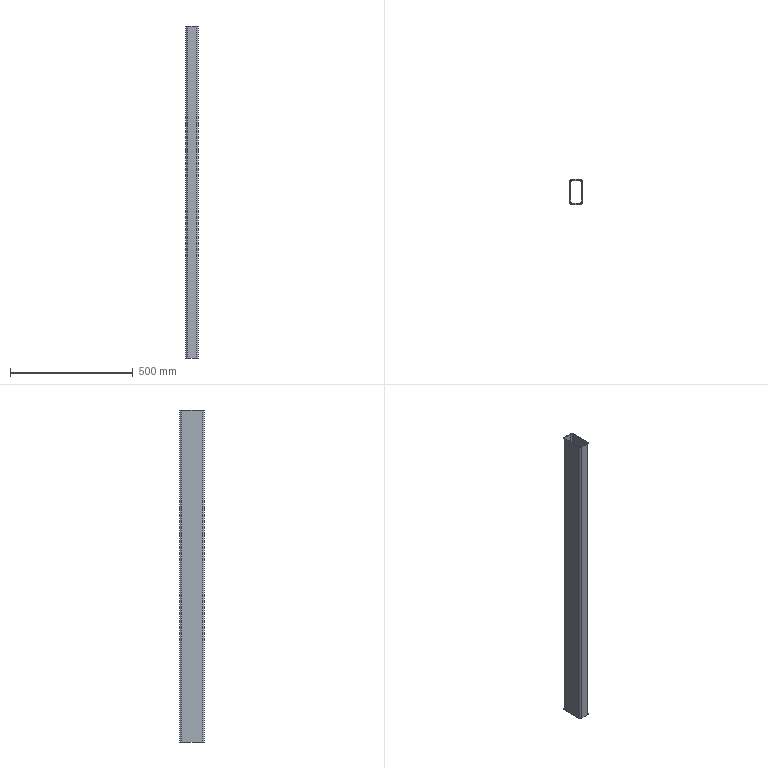Part | STEP file | KS D 3568 - 100 x 50 x 3.2 - 1350 | 1 solid | 18 faces | box 50 x 100 x 1350 mm | volume 1193238 mm3 | plane 10 | cylinder 8 | commonest cylinder face diameters 9.6 x4 16 x4
STEP:
#1=CARTESIAN_POINT('',(0.,0.,0.));
#2=DIRECTION('',(0.,0.,1.));
#3=DIRECTION('',(1.,0.,0.));
#4=AXIS2_PLACEMENT_3D('',#1,#2,#3);
#5=CARTESIAN_POINT('',(17.,46.8,1400.));
#6=VERTEX_POINT('',#5);
#7=CARTESIAN_POINT('',(-17.,46.8,1400.));
#8=VERTEX_POINT('',#7);
#9=CARTESIAN_POINT('',(-8.5,46.8,1400.));
#10=DIRECTION('',(-1.,0.,0.));
#11=VECTOR('',#10,1.);
#12=LINE('',#9,#11);
#13=CARTESIAN_POINT('',(0.,0.,1400.));
#14=DIRECTION('',(0.,0.,1.));
#15=DIRECTION('',(1.,0.,0.));
#16=AXIS2_PLACEMENT_3D('',#13,#14,#15);
#17=PLANE('',#16);
#18=CARTESIAN_POINT('',(-8.5,46.8));
#19=DIRECTION('',(-1.,0.));
#20=VECTOR('',#19,1.);
#21=LINE('',#18,#20);
#22=(GEOMETRIC_REPRESENTATION_CONTEXT(2)PARAMETRIC_REPRESENTATION_CONTEXT()REPRESENTATION_CONTEXT('',''));
#23=DEFINITIONAL_REPRESENTATION('',(#21),#22);
#24=PCURVE('',#17,#23);
#25=CARTESIAN_POINT('',(-17.,46.8,0.));
#26=DIRECTION('',(0.,1.,0.));
#27=DIRECTION('',(1.,0.,0.));
#28=AXIS2_PLACEMENT_3D('',#25,#26,#27);
#29=PLANE('',#28);
#30=CARTESIAN_POINT('',(8.5,-1400.));
#31=DIRECTION('',(-1.,0.));
#32=VECTOR('',#31,1.);
#33=LINE('',#30,#32);
#34=(GEOMETRIC_REPRESENTATION_CONTEXT(2)PARAMETRIC_REPRESENTATION_CONTEXT()REPRESENTATION_CONTEXT('',''));
#35=DEFINITIONAL_REPRESENTATION('',(#33),#34);
#36=PCURVE('',#29,#35);
#37=SURFACE_CURVE('',#12,(#24,#36),.PCURVE_S1.);
#38=EDGE_CURVE('',#6,#8,#37,.T.);
#39=ORIENTED_EDGE('',*,*,#38,.F.);
#40=CARTESIAN_POINT('',(21.8,42.,1400.));
#41=VERTEX_POINT('',#40);
#42=CARTESIAN_POINT('',(17.,42.,1400.));
#43=DIRECTION('',(0.,0.,1.));
#44=DIRECTION('',(-1.,0.,0.));
#45=AXIS2_PLACEMENT_3D('',#42,#43,#44);
#46=CIRCLE('',#45,4.8);
#47=CARTESIAN_POINT('',(17.,42.));
#48=DIRECTION('',(-1.,0.));
#49=AXIS2_PLACEMENT_2D('',#47,#48);
#50=CIRCLE('',#49,4.8);
#51=(GEOMETRIC_REPRESENTATION_CONTEXT(2)PARAMETRIC_REPRESENTATION_CONTEXT()REPRESENTATION_CONTEXT('',''));
#52=DEFINITIONAL_REPRESENTATION('',(#50),#51);
#53=PCURVE('',#17,#52);
#54=CARTESIAN_POINT('',(17.,42.,0.));
#55=DIRECTION('',(0.,0.,1.));
#56=DIRECTION('',(-1.,0.,0.));
#57=AXIS2_PLACEMENT_3D('',#54,#55,#56);
#58=CYLINDRICAL_SURFACE('',#57,4.8);
#59=CARTESIAN_POINT('',(0.,1400.));
#60=DIRECTION('',(1.,0.));
#61=VECTOR('',#60,1.);
#62=LINE('',#59,#61);
#63=(GEOMETRIC_REPRESENTATION_CONTEXT(2)PARAMETRIC_REPRESENTATION_CONTEXT()REPRESENTATION_CONTEXT('',''));
#64=DEFINITIONAL_REPRESENTATION('',(#62),#63);
#65=PCURVE('',#58,#64);
#66=SURFACE_CURVE('',#46,(#53,#65),.PCURVE_S1.);
#67=EDGE_CURVE('',#41,#6,#66,.T.);
#68=ORIENTED_EDGE('',*,*,#67,.F.);
#69=CARTESIAN_POINT('',(21.8,-42.,1400.));
#70=VERTEX_POINT('',#69);
#71=CARTESIAN_POINT('',(21.8,21.,1400.));
#72=DIRECTION('',(0.,1.,0.));
#73=VECTOR('',#72,1.);
#74=LINE('',#71,#73);
#75=CARTESIAN_POINT('',(21.8,21.));
#76=DIRECTION('',(0.,1.));
#77=VECTOR('',#76,1.);
#78=LINE('',#75,#77);
#79=(GEOMETRIC_REPRESENTATION_CONTEXT(2)PARAMETRIC_REPRESENTATION_CONTEXT()REPRESENTATION_CONTEXT('',''));
#80=DEFINITIONAL_REPRESENTATION('',(#78),#79);
#81=PCURVE('',#17,#80);
#82=CARTESIAN_POINT('',(21.8,42.,0.));
#83=DIRECTION('',(1.,0.,0.));
#84=DIRECTION('',(0.,1.,0.));
#85=AXIS2_PLACEMENT_3D('',#82,#83,#84);
#86=PLANE('',#85);
#87=CARTESIAN_POINT('',(-21.,1400.));
#88=DIRECTION('',(1.,0.));
#89=VECTOR('',#88,1.);
#90=LINE('',#87,#89);
#91=(GEOMETRIC_REPRESENTATION_CONTEXT(2)PARAMETRIC_REPRESENTATION_CONTEXT()REPRESENTATION_CONTEXT('',''));
#92=DEFINITIONAL_REPRESENTATION('',(#90),#91);
#93=PCURVE('',#86,#92);
#94=SURFACE_CURVE('',#74,(#81,#93),.PCURVE_S1.);
#95=EDGE_CURVE('',#70,#41,#94,.T.);
#96=ORIENTED_EDGE('',*,*,#95,.F.);
#97=CARTESIAN_POINT('',(17.,-46.8,1400.));
#98=VERTEX_POINT('',#97);
#99=CARTESIAN_POINT('',(17.,-42.,1400.));
#100=DIRECTION('',(0.,0.,1.));
#101=DIRECTION('',(0.,1.,0.));
#102=AXIS2_PLACEMENT_3D('',#99,#100,#101);
#103=CIRCLE('',#102,4.8);
#104=CARTESIAN_POINT('',(17.,-42.));
#105=DIRECTION('',(0.,1.));
#106=AXIS2_PLACEMENT_2D('',#104,#105);
#107=CIRCLE('',#106,4.8);
#108=(GEOMETRIC_REPRESENTATION_CONTEXT(2)PARAMETRIC_REPRESENTATION_CONTEXT()REPRESENTATION_CONTEXT('',''));
#109=DEFINITIONAL_REPRESENTATION('',(#107),#108);
#110=PCURVE('',#17,#109);
#111=CARTESIAN_POINT('',(17.,-42.,0.));
#112=DIRECTION('',(0.,0.,1.));
#113=DIRECTION('',(0.,1.,0.));
#114=AXIS2_PLACEMENT_3D('',#111,#112,#113);
#115=CYLINDRICAL_SURFACE('',#114,4.8);
#116=CARTESIAN_POINT('',(0.,1400.));
#117=DIRECTION('',(1.,0.));
#118=VECTOR('',#117,1.);
#119=LINE('',#116,#118);
#120=(GEOMETRIC_REPRESENTATION_CONTEXT(2)PARAMETRIC_REPRESENTATION_CONTEXT()REPRESENTATION_CONTEXT('',''));
#121=DEFINITIONAL_REPRESENTATION('',(#119),#120);
#122=PCURVE('',#115,#121);
#123=SURFACE_CURVE('',#103,(#110,#122),.PCURVE_S1.);
#124=EDGE_CURVE('',#98,#70,#123,.T.);
#125=ORIENTED_EDGE('',*,*,#124,.F.);
#126=CARTESIAN_POINT('',(-17.,-46.8,1400.));
#127=VERTEX_POINT('',#126);
#128=CARTESIAN_POINT('',(8.5,-46.8,1400.));
#129=DIRECTION('',(1.,0.,0.));
#130=VECTOR('',#129,1.);
#131=LINE('',#128,#130);
#132=CARTESIAN_POINT('',(8.5,-46.8));
#133=DIRECTION('',(1.,0.));
#134=VECTOR('',#133,1.);
#135=LINE('',#132,#134);
#136=(GEOMETRIC_REPRESENTATION_CONTEXT(2)PARAMETRIC_REPRESENTATION_CONTEXT()REPRESENTATION_CONTEXT('',''));
#137=DEFINITIONAL_REPRESENTATION('',(#135),#136);
#138=PCURVE('',#17,#137);
#139=CARTESIAN_POINT('',(17.,-46.8,0.));
#140=DIRECTION('',(0.,-1.,0.));
#141=DIRECTION('',(0.,0.,-1.));
#142=AXIS2_PLACEMENT_3D('',#139,#140,#141);
#143=PLANE('',#142);
#144=CARTESIAN_POINT('',(-1400.,-8.5));
#145=DIRECTION('',(0.,1.));
#146=VECTOR('',#145,1.);
#147=LINE('',#144,#146);
#148=(GEOMETRIC_REPRESENTATION_CONTEXT(2)PARAMETRIC_REPRESENTATION_CONTEXT()REPRESENTATION_CONTEXT('',''));
#149=DEFINITIONAL_REPRESENTATION('',(#147),#148);
#150=PCURVE('',#143,#149);
#151=SURFACE_CURVE('',#131,(#138,#150),.PCURVE_S1.);
#152=EDGE_CURVE('',#127,#98,#151,.T.);
#153=ORIENTED_EDGE('',*,*,#152,.F.);
#154=CARTESIAN_POINT('',(-21.8,-42.,1400.));
#155=VERTEX_POINT('',#154);
#156=CARTESIAN_POINT('',(-17.,-42.,1400.));
#157=DIRECTION('',(0.,0.,1.));
#158=DIRECTION('',(1.,0.,0.));
#159=AXIS2_PLACEMENT_3D('',#156,#157,#158);
#160=CIRCLE('',#159,4.8);
#161=CARTESIAN_POINT('',(-17.,-42.));
#162=DIRECTION('',(1.,0.));
#163=AXIS2_PLACEMENT_2D('',#161,#162);
#164=CIRCLE('',#163,4.8);
#165=(GEOMETRIC_REPRESENTATION_CONTEXT(2)PARAMETRIC_REPRESENTATION_CONTEXT()REPRESENTATION_CONTEXT('',''));
#166=DEFINITIONAL_REPRESENTATION('',(#164),#165);
#167=PCURVE('',#17,#166);
#168=CARTESIAN_POINT('',(-17.,-42.,0.));
#169=DIRECTION('',(0.,0.,1.));
#170=DIRECTION('',(1.,0.,0.));
#171=AXIS2_PLACEMENT_3D('',#168,#169,#170);
#172=CYLINDRICAL_SURFACE('',#171,4.8);
#173=CARTESIAN_POINT('',(0.,1400.));
#174=DIRECTION('',(1.,0.));
#175=VECTOR('',#174,1.);
#176=LINE('',#173,#175);
#177=(GEOMETRIC_REPRESENTATION_CONTEXT(2)PARAMETRIC_REPRESENTATION_CONTEXT()REPRESENTATION_CONTEXT('',''));
#178=DEFINITIONAL_REPRESENTATION('',(#176),#177);
#179=PCURVE('',#172,#178);
#180=SURFACE_CURVE('',#160,(#167,#179),.PCURVE_S1.);
#181=EDGE_CURVE('',#155,#127,#180,.T.);
#182=ORIENTED_EDGE('',*,*,#181,.F.);
#183=CARTESIAN_POINT('',(-21.8,42.,1400.));
#184=VERTEX_POINT('',#183);
#185=CARTESIAN_POINT('',(-21.8,-21.,1400.));
#186=DIRECTION('',(0.,-1.,0.));
#187=VECTOR('',#186,1.);
#188=LINE('',#185,#187);
#189=CARTESIAN_POINT('',(-21.8,-21.));
#190=DIRECTION('',(0.,-1.));
#191=VECTOR('',#190,1.);
#192=LINE('',#189,#191);
#193=(GEOMETRIC_REPRESENTATION_CONTEXT(2)PARAMETRIC_REPRESENTATION_CONTEXT()REPRESENTATION_CONTEXT('',''));
#194=DEFINITIONAL_REPRESENTATION('',(#192),#193);
#195=PCURVE('',#17,#194);
#196=CARTESIAN_POINT('',(-21.8,-42.,0.));
#197=DIRECTION('',(-1.,0.,0.));
#198=DIRECTION('',(0.,1.,0.));
#199=AXIS2_PLACEMENT_3D('',#196,#197,#198);
#200=PLANE('',#199);
#201=CARTESIAN_POINT('',(21.,-1400.));
#202=DIRECTION('',(-1.,0.));
#203=VECTOR('',#202,1.);
#204=LINE('',#201,#203);
#205=(GEOMETRIC_REPRESENTATION_CONTEXT(2)PARAMETRIC_REPRESENTATION_CONTEXT()REPRESENTATION_CONTEXT('',''));
#206=DEFINITIONAL_REPRESENTATION('',(#204),#205);
#207=PCURVE('',#200,#206);
#208=SURFACE_CURVE('',#188,(#195,#207),.PCURVE_S1.);
#209=EDGE_CURVE('',#184,#155,#208,.T.);
#210=ORIENTED_EDGE('',*,*,#209,.F.);
#211=CARTESIAN_POINT('',(-17.,42.,1400.));
#212=DIRECTION('',(0.,0.,1.));
#213=DIRECTION('',(0.,-1.,0.));
#214=AXIS2_PLACEMENT_3D('',#211,#212,#213);
#215=CIRCLE('',#214,4.8);
#216=CARTESIAN_POINT('',(-17.,42.));
#217=DIRECTION('',(0.,-1.));
#218=AXIS2_PLACEMENT_2D('',#216,#217);
#219=CIRCLE('',#218,4.8);
#220=(GEOMETRIC_REPRESENTATION_CONTEXT(2)PARAMETRIC_REPRESENTATION_CONTEXT()REPRESENTATION_CONTEXT('',''));
#221=DEFINITIONAL_REPRESENTATION('',(#219),#220);
#222=PCURVE('',#17,#221);
#223=CARTESIAN_POINT('',(-17.,42.,0.));
#224=DIRECTION('',(0.,0.,1.));
#225=DIRECTION('',(0.,-1.,0.));
#226=AXIS2_PLACEMENT_3D('',#223,#224,#225);
#227=CYLINDRICAL_SURFACE('',#226,4.8);
#228=CARTESIAN_POINT('',(0.,1400.));
#229=DIRECTION('',(1.,0.));
#230=VECTOR('',#229,1.);
#231=LINE('',#228,#230);
#232=(GEOMETRIC_REPRESENTATION_CONTEXT(2)PARAMETRIC_REPRESENTATION_CONTEXT()REPRESENTATION_CONTEXT('',''));
#233=DEFINITIONAL_REPRESENTATION('',(#231),#232);
#234=PCURVE('',#227,#233);
#235=SURFACE_CURVE('',#215,(#222,#234),.PCURVE_S1.);
#236=EDGE_CURVE('',#8,#184,#235,.T.);
#237=ORIENTED_EDGE('',*,*,#236,.F.);
#238=EDGE_LOOP('',(#39,#68,#96,#125,#153,#182,#210,#237));
#239=FACE_BOUND('',#238,.T.);
#240=CARTESIAN_POINT('',(-25.,-42.,1400.));
#241=VERTEX_POINT('',#240);
#242=CARTESIAN_POINT('',(-25.,42.,1400.));
#243=VERTEX_POINT('',#242);
#244=CARTESIAN_POINT('',(-25.,-21.,1400.));
#245=DIRECTION('',(0.,1.,0.));
#246=VECTOR('',#245,1.);
#247=LINE('',#244,#246);
#248=CARTESIAN_POINT('',(-25.,-21.));
#249=DIRECTION('',(0.,1.));
#250=VECTOR('',#249,1.);
#251=LINE('',#248,#250);
#252=(GEOMETRIC_REPRESENTATION_CONTEXT(2)PARAMETRIC_REPRESENTATION_CONTEXT()REPRESENTATION_CONTEXT('',''));
#253=DEFINITIONAL_REPRESENTATION('',(#251),#252);
#254=PCURVE('',#17,#253);
#255=CARTESIAN_POINT('',(-25.,-42.,0.));
#256=DIRECTION('',(-1.,0.,0.));
#257=DIRECTION('',(0.,1.,0.));
#258=AXIS2_PLACEMENT_3D('',#255,#256,#257);
#259=PLANE('',#258);
#260=CARTESIAN_POINT('',(21.,-1400.));
#261=DIRECTION('',(1.,0.));
#262=VECTOR('',#261,1.);
#263=LINE('',#260,#262);
#264=(GEOMETRIC_REPRESENTATION_CONTEXT(2)PARAMETRIC_REPRESENTATION_CONTEXT()REPRESENTATION_CONTEXT('',''));
#265=DEFINITIONAL_REPRESENTATION('',(#263),#264);
#266=PCURVE('',#259,#265);
#267=SURFACE_CURVE('',#247,(#254,#266),.PCURVE_S1.);
#268=EDGE_CURVE('',#241,#243,#267,.T.);
#269=ORIENTED_EDGE('',*,*,#268,.F.);
#270=CARTESIAN_POINT('',(-17.,-50.,1400.));
#271=VERTEX_POINT('',#270);
#272=CARTESIAN_POINT('',(-17.,-42.,1400.));
#273=DIRECTION('',(0.,0.,-1.));
#274=DIRECTION('',(1.,0.,0.));
#275=AXIS2_PLACEMENT_3D('',#272,#273,#274);
#276=CIRCLE('',#275,8.);
#277=CARTESIAN_POINT('',(-9.,-42.));
#278=CARTESIAN_POINT('',(-9.,-55.856));
#279=CARTESIAN_POINT('',(-21.,-48.928));
#280=CARTESIAN_POINT('',(-33.,-42.));
#281=CARTESIAN_POINT('',(-21.,-35.072));
#282=CARTESIAN_POINT('',(-9.,-28.144));
#283=CARTESIAN_POINT('',(-9.,-42.));
#284=(BOUNDED_CURVE()B_SPLINE_CURVE(2,(#277,#278,#279,#280,#281,#282,#283),.UNSPECIFIED.,.T.,.F.)B_SPLINE_CURVE_WITH_KNOTS((1,2,2,2,2,1),(-2.094,0.,2.094,4.189,6.283,8.378),.UNSPECIFIED.)CURVE()GEOMETRIC_REPRESENTATION_ITEM()RATIONAL_B_SPLINE_CURVE((1.,0.5,1.,0.5,1.,0.5,1.))REPRESENTATION_ITEM(''));
#285=(GEOMETRIC_REPRESENTATION_CONTEXT(2)PARAMETRIC_REPRESENTATION_CONTEXT()REPRESENTATION_CONTEXT('',''));
#286=DEFINITIONAL_REPRESENTATION('',(#284),#285);
#287=PCURVE('',#17,#286);
#288=CARTESIAN_POINT('',(-17.,-42.,0.));
#289=DIRECTION('',(0.,0.,1.));
#290=DIRECTION('',(1.,0.,0.));
#291=AXIS2_PLACEMENT_3D('',#288,#289,#290);
#292=CYLINDRICAL_SURFACE('',#291,8.);
#293=CARTESIAN_POINT('',(6.283,1400.));
#294=DIRECTION('',(-1.,0.));
#295=VECTOR('',#294,1.);
#296=LINE('',#293,#295);
#297=(GEOMETRIC_REPRESENTATION_CONTEXT(2)PARAMETRIC_REPRESENTATION_CONTEXT()REPRESENTATION_CONTEXT('',''));
#298=DEFINITIONAL_REPRESENTATION('',(#296),#297);
#299=PCURVE('',#292,#298);
#300=SURFACE_CURVE('',#276,(#287,#299),.PCURVE_S1.);
#301=EDGE_CURVE('',#271,#241,#300,.T.);
#302=ORIENTED_EDGE('',*,*,#301,.F.);
#303=CARTESIAN_POINT('',(17.,-50.,1400.));
#304=VERTEX_POINT('',#303);
#305=CARTESIAN_POINT('',(8.5,-50.,1400.));
#306=DIRECTION('',(-1.,0.,0.));
#307=VECTOR('',#306,1.);
#308=LINE('',#305,#307);
#309=CARTESIAN_POINT('',(8.5,-50.));
#310=DIRECTION('',(-1.,0.));
#311=VECTOR('',#310,1.);
#312=LINE('',#309,#311);
#313=(GEOMETRIC_REPRESENTATION_CONTEXT(2)PARAMETRIC_REPRESENTATION_CONTEXT()REPRESENTATION_CONTEXT('',''));
#314=DEFINITIONAL_REPRESENTATION('',(#312),#313);
#315=PCURVE('',#17,#314);
#316=CARTESIAN_POINT('',(17.,-50.,0.));
#317=DIRECTION('',(0.,-1.,0.));
#318=DIRECTION('',(-1.,0.,0.));
#319=AXIS2_PLACEMENT_3D('',#316,#317,#318);
#320=PLANE('',#319);
#321=CARTESIAN_POINT('',(8.5,-1400.));
#322=DIRECTION('',(1.,0.));
#323=VECTOR('',#322,1.);
#324=LINE('',#321,#323);
#325=(GEOMETRIC_REPRESENTATION_CONTEXT(2)PARAMETRIC_REPRESENTATION_CONTEXT()REPRESENTATION_CONTEXT('',''));
#326=DEFINITIONAL_REPRESENTATION('',(#324),#325);
#327=PCURVE('',#320,#326);
#328=SURFACE_CURVE('',#308,(#315,#327),.PCURVE_S1.);
#329=EDGE_CURVE('',#304,#271,#328,.T.);
#330=ORIENTED_EDGE('',*,*,#329,.F.);
#331=CARTESIAN_POINT('',(25.,-42.,1400.));
#332=VERTEX_POINT('',#331);
#333=CARTESIAN_POINT('',(17.,-42.,1400.));
#334=DIRECTION('',(0.,0.,-1.));
#335=DIRECTION('',(0.,1.,0.));
#336=AXIS2_PLACEMENT_3D('',#333,#334,#335);
#337=CIRCLE('',#336,8.);
#338=CARTESIAN_POINT('',(17.,-34.));
#339=CARTESIAN_POINT('',(30.856,-34.));
#340=CARTESIAN_POINT('',(23.928,-46.));
#341=CARTESIAN_POINT('',(17.,-58.));
#342=CARTESIAN_POINT('',(10.072,-46.));
#343=CARTESIAN_POINT('',(3.144,-34.));
#344=CARTESIAN_POINT('',(17.,-34.));
#345=(BOUNDED_CURVE()B_SPLINE_CURVE(2,(#338,#339,#340,#341,#342,#343,#344),.UNSPECIFIED.,.T.,.F.)B_SPLINE_CURVE_WITH_KNOTS((1,2,2,2,2,1),(-2.094,0.,2.094,4.189,6.283,8.378),.UNSPECIFIED.)CURVE()GEOMETRIC_REPRESENTATION_ITEM()RATIONAL_B_SPLINE_CURVE((1.,0.5,1.,0.5,1.,0.5,1.))REPRESENTATION_ITEM(''));
#346=(GEOMETRIC_REPRESENTATION_CONTEXT(2)PARAMETRIC_REPRESENTATION_CONTEXT()REPRESENTATION_CONTEXT('',''));
#347=DEFINITIONAL_REPRESENTATION('',(#345),#346);
#348=PCURVE('',#17,#347);
#349=CARTESIAN_POINT('',(17.,-42.,0.));
#350=DIRECTION('',(0.,0.,1.));
#351=DIRECTION('',(0.,1.,0.));
#352=AXIS2_PLACEMENT_3D('',#349,#350,#351);
#353=CYLINDRICAL_SURFACE('',#352,8.);
#354=CARTESIAN_POINT('',(6.283,1400.));
#355=DIRECTION('',(-1.,0.));
#356=VECTOR('',#355,1.);
#357=LINE('',#354,#356);
#358=(GEOMETRIC_REPRESENTATION_CONTEXT(2)PARAMETRIC_REPRESENTATION_CONTEXT()REPRESENTATION_CONTEXT('',''));
#359=DEFINITIONAL_REPRESENTATION('',(#357),#358);
#360=PCURVE('',#353,#359);
#361=SURFACE_CURVE('',#337,(#348,#360),.PCURVE_S1.);
#362=EDGE_CURVE('',#332,#304,#361,.T.);
#363=ORIENTED_EDGE('',*,*,#362,.F.);
#364=CARTESIAN_POINT('',(25.,42.,1400.));
#365=VERTEX_POINT('',#364);
#366=CARTESIAN_POINT('',(25.,21.,1400.));
#367=DIRECTION('',(0.,-1.,0.));
#368=VECTOR('',#367,1.);
#369=LINE('',#366,#368);
#370=CARTESIAN_POINT('',(25.,21.));
#371=DIRECTION('',(0.,-1.));
#372=VECTOR('',#371,1.);
#373=LINE('',#370,#372);
#374=(GEOMETRIC_REPRESENTATION_CONTEXT(2)PARAMETRIC_REPRESENTATION_CONTEXT()REPRESENTATION_CONTEXT('',''));
#375=DEFINITIONAL_REPRESENTATION('',(#373),#374);
#376=PCURVE('',#17,#375);
#377=CARTESIAN_POINT('',(25.,42.,0.));
#378=DIRECTION('',(1.,0.,0.));
#379=DIRECTION('',(0.,-1.,0.));
#380=AXIS2_PLACEMENT_3D('',#377,#378,#379);
#381=PLANE('',#380);
#382=CARTESIAN_POINT('',(21.,-1400.));
#383=DIRECTION('',(1.,0.));
#384=VECTOR('',#383,1.);
#385=LINE('',#382,#384);
#386=(GEOMETRIC_REPRESENTATION_CONTEXT(2)PARAMETRIC_REPRESENTATION_CONTEXT()REPRESENTATION_CONTEXT('',''));
#387=DEFINITIONAL_REPRESENTATION('',(#385),#386);
#388=PCURVE('',#381,#387);
#389=SURFACE_CURVE('',#369,(#376,#388),.PCURVE_S1.);
#390=EDGE_CURVE('',#365,#332,#389,.T.);
#391=ORIENTED_EDGE('',*,*,#390,.F.);
#392=CARTESIAN_POINT('',(17.,50.,1400.));
#393=VERTEX_POINT('',#392);
#394=CARTESIAN_POINT('',(17.,42.,1400.));
#395=DIRECTION('',(0.,0.,-1.));
#396=DIRECTION('',(-1.,0.,0.));
#397=AXIS2_PLACEMENT_3D('',#394,#395,#396);
#398=CIRCLE('',#397,8.);
#399=CARTESIAN_POINT('',(9.,42.));
#400=CARTESIAN_POINT('',(9.,55.856));
#401=CARTESIAN_POINT('',(21.,48.928));
#402=CARTESIAN_POINT('',(33.,42.));
#403=CARTESIAN_POINT('',(21.,35.072));
#404=CARTESIAN_POINT('',(9.,28.144));
#405=CARTESIAN_POINT('',(9.,42.));
#406=(BOUNDED_CURVE()B_SPLINE_CURVE(2,(#399,#400,#401,#402,#403,#404,#405),.UNSPECIFIED.,.T.,.F.)B_SPLINE_CURVE_WITH_KNOTS((1,2,2,2,2,1),(-2.094,0.,2.094,4.189,6.283,8.378),.UNSPECIFIED.)CURVE()GEOMETRIC_REPRESENTATION_ITEM()RATIONAL_B_SPLINE_CURVE((1.,0.5,1.,0.5,1.,0.5,1.))REPRESENTATION_ITEM(''));
#407=(GEOMETRIC_REPRESENTATION_CONTEXT(2)PARAMETRIC_REPRESENTATION_CONTEXT()REPRESENTATION_CONTEXT('',''));
#408=DEFINITIONAL_REPRESENTATION('',(#406),#407);
#409=PCURVE('',#17,#408);
#410=CARTESIAN_POINT('',(17.,42.,0.));
#411=DIRECTION('',(0.,0.,1.));
#412=DIRECTION('',(-1.,0.,0.));
#413=AXIS2_PLACEMENT_3D('',#410,#411,#412);
#414=CYLINDRICAL_SURFACE('',#413,8.);
#415=CARTESIAN_POINT('',(6.283,1400.));
#416=DIRECTION('',(-1.,0.));
#417=VECTOR('',#416,1.);
#418=LINE('',#415,#417);
#419=(GEOMETRIC_REPRESENTATION_CONTEXT(2)PARAMETRIC_REPRESENTATION_CONTEXT()REPRESENTATION_CONTEXT('',''));
#420=DEFINITIONAL_REPRESENTATION('',(#418),#419);
#421=PCURVE('',#414,#420);
#422=SURFACE_CURVE('',#398,(#409,#421),.PCURVE_S1.);
#423=EDGE_CURVE('',#393,#365,#422,.T.);
#424=ORIENTED_EDGE('',*,*,#423,.F.);
#425=CARTESIAN_POINT('',(-17.,50.,1400.));
#426=VERTEX_POINT('',#425);
#427=CARTESIAN_POINT('',(-8.5,50.,1400.));
#428=DIRECTION('',(1.,0.,0.));
#429=VECTOR('',#428,1.);
#430=LINE('',#427,#429);
#431=CARTESIAN_POINT('',(-8.5,50.));
#432=DIRECTION('',(1.,0.));
#433=VECTOR('',#432,1.);
#434=LINE('',#431,#433);
#435=(GEOMETRIC_REPRESENTATION_CONTEXT(2)PARAMETRIC_REPRESENTATION_CONTEXT()REPRESENTATION_CONTEXT('',''));
#436=DEFINITIONAL_REPRESENTATION('',(#434),#435);
#437=PCURVE('',#17,#436);
#438=CARTESIAN_POINT('',(-17.,50.,0.));
#439=DIRECTION('',(0.,1.,0.));
#440=DIRECTION('',(1.,0.,0.));
#441=AXIS2_PLACEMENT_3D('',#438,#439,#440);
#442=PLANE('',#441);
#443=CARTESIAN_POINT('',(8.5,-1400.));
#444=DIRECTION('',(1.,0.));
#445=VECTOR('',#444,1.);
#446=LINE('',#443,#445);
#447=(GEOMETRIC_REPRESENTATION_CONTEXT(2)PARAMETRIC_REPRESENTATION_CONTEXT()REPRESENTATION_CONTEXT('',''));
#448=DEFINITIONAL_REPRESENTATION('',(#446),#447);
#449=PCURVE('',#442,#448);
#450=SURFACE_CURVE('',#430,(#437,#449),.PCURVE_S1.);
#451=EDGE_CURVE('',#426,#393,#450,.T.);
#452=ORIENTED_EDGE('',*,*,#451,.F.);
#453=CARTESIAN_POINT('',(-17.,42.,1400.));
#454=DIRECTION('',(0.,0.,-1.));
#455=DIRECTION('',(0.,-1.,0.));
#456=AXIS2_PLACEMENT_3D('',#453,#454,#455);
#457=CIRCLE('',#456,8.);
#458=CARTESIAN_POINT('',(-17.,34.));
#459=CARTESIAN_POINT('',(-30.856,34.));
#460=CARTESIAN_POINT('',(-23.928,46.));
#461=CARTESIAN_POINT('',(-17.,58.));
#462=CARTESIAN_POINT('',(-10.072,46.));
#463=CARTESIAN_POINT('',(-3.144,34.));
#464=CARTESIAN_POINT('',(-17.,34.));
#465=(BOUNDED_CURVE()B_SPLINE_CURVE(2,(#458,#459,#460,#461,#462,#463,#464),.UNSPECIFIED.,.T.,.F.)B_SPLINE_CURVE_WITH_KNOTS((1,2,2,2,2,1),(-2.094,0.,2.094,4.189,6.283,8.378),.UNSPECIFIED.)CURVE()GEOMETRIC_REPRESENTATION_ITEM()RATIONAL_B_SPLINE_CURVE((1.,0.5,1.,0.5,1.,0.5,1.))REPRESENTATION_ITEM(''));
#466=(GEOMETRIC_REPRESENTATION_CONTEXT(2)PARAMETRIC_REPRESENTATION_CONTEXT()REPRESENTATION_CONTEXT('',''));
#467=DEFINITIONAL_REPRESENTATION('',(#465),#466);
#468=PCURVE('',#17,#467);
#469=CARTESIAN_POINT('',(-17.,42.,0.));
#470=DIRECTION('',(0.,0.,1.));
#471=DIRECTION('',(0.,-1.,0.));
#472=AXIS2_PLACEMENT_3D('',#469,#470,#471);
#473=CYLINDRICAL_SURFACE('',#472,8.);
#474=CARTESIAN_POINT('',(6.283,1400.));
#475=DIRECTION('',(-1.,0.));
#476=VECTOR('',#475,1.);
#477=LINE('',#474,#476);
#478=(GEOMETRIC_REPRESENTATION_CONTEXT(2)PARAMETRIC_REPRESENTATION_CONTEXT()REPRESENTATION_CONTEXT('',''));
#479=DEFINITIONAL_REPRESENTATION('',(#477),#478);
#480=PCURVE('',#473,#479);
#481=SURFACE_CURVE('',#457,(#468,#480),.PCURVE_S1.);
#482=EDGE_CURVE('',#243,#426,#481,.T.);
#483=ORIENTED_EDGE('',*,*,#482,.F.);
#484=EDGE_LOOP('',(#269,#302,#330,#363,#391,#424,#452,#483));
#485=FACE_BOUND('',#484,.T.);
#486=ADVANCED_FACE('',(#239,#485),#17,.T.);
#487=CARTESIAN_POINT('',(17.,46.8,50.));
#488=VERTEX_POINT('',#487);
#489=CARTESIAN_POINT('',(-17.,46.8,50.));
#490=VERTEX_POINT('',#489);
#491=CARTESIAN_POINT('',(-8.5,46.8,50.));
#492=DIRECTION('',(-1.,0.,0.));
#493=VECTOR('',#492,1.);
#494=LINE('',#491,#493);
#495=CARTESIAN_POINT('',(0.,0.,50.));
#496=DIRECTION('',(0.,0.,1.));
#497=DIRECTION('',(1.,0.,0.));
#498=AXIS2_PLACEMENT_3D('',#495,#496,#497);
#499=PLANE('',#498);
#500=CARTESIAN_POINT('',(-8.5,46.8));
#501=DIRECTION('',(-1.,0.));
#502=VECTOR('',#501,1.);
#503=LINE('',#500,#502);
#504=(GEOMETRIC_REPRESENTATION_CONTEXT(2)PARAMETRIC_REPRESENTATION_CONTEXT()REPRESENTATION_CONTEXT('',''));
#505=DEFINITIONAL_REPRESENTATION('',(#503),#504);
#506=PCURVE('',#499,#505);
#507=CARTESIAN_POINT('',(8.5,-50.));
#508=DIRECTION('',(-1.,0.));
#509=VECTOR('',#508,1.);
#510=LINE('',#507,#509);
#511=(GEOMETRIC_REPRESENTATION_CONTEXT(2)PARAMETRIC_REPRESENTATION_CONTEXT()REPRESENTATION_CONTEXT('',''));
#512=DEFINITIONAL_REPRESENTATION('',(#510),#511);
#513=PCURVE('',#29,#512);
#514=SURFACE_CURVE('',#494,(#506,#513),.PCURVE_S1.);
#515=EDGE_CURVE('',#488,#490,#514,.T.);
#516=ORIENTED_EDGE('',*,*,#515,.T.);
#517=CARTESIAN_POINT('',(-21.8,42.,50.));
#518=VERTEX_POINT('',#517);
#519=CARTESIAN_POINT('',(-17.,42.,50.));
#520=DIRECTION('',(0.,0.,1.));
#521=DIRECTION('',(0.,-1.,0.));
#522=AXIS2_PLACEMENT_3D('',#519,#520,#521);
#523=CIRCLE('',#522,4.8);
#524=CARTESIAN_POINT('',(-17.,42.));
#525=DIRECTION('',(0.,-1.));
#526=AXIS2_PLACEMENT_2D('',#524,#525);
#527=CIRCLE('',#526,4.8);
#528=(GEOMETRIC_REPRESENTATION_CONTEXT(2)PARAMETRIC_REPRESENTATION_CONTEXT()REPRESENTATION_CONTEXT('',''));
#529=DEFINITIONAL_REPRESENTATION('',(#527),#528);
#530=PCURVE('',#499,#529);
#531=CARTESIAN_POINT('',(0.,50.));
#532=DIRECTION('',(1.,0.));
#533=VECTOR('',#532,1.);
#534=LINE('',#531,#533);
#535=(GEOMETRIC_REPRESENTATION_CONTEXT(2)PARAMETRIC_REPRESENTATION_CONTEXT()REPRESENTATION_CONTEXT('',''));
#536=DEFINITIONAL_REPRESENTATION('',(#534),#535);
#537=PCURVE('',#227,#536);
#538=SURFACE_CURVE('',#523,(#530,#537),.PCURVE_S1.);
#539=EDGE_CURVE('',#490,#518,#538,.T.);
#540=ORIENTED_EDGE('',*,*,#539,.T.);
#541=CARTESIAN_POINT('',(-21.8,-42.,50.));
#542=VERTEX_POINT('',#541);
#543=CARTESIAN_POINT('',(-21.8,-21.,50.));
#544=DIRECTION('',(0.,-1.,0.));
#545=VECTOR('',#544,1.);
#546=LINE('',#543,#545);
#547=CARTESIAN_POINT('',(-21.8,-21.));
#548=DIRECTION('',(0.,-1.));
#549=VECTOR('',#548,1.);
#550=LINE('',#547,#549);
#551=(GEOMETRIC_REPRESENTATION_CONTEXT(2)PARAMETRIC_REPRESENTATION_CONTEXT()REPRESENTATION_CONTEXT('',''));
#552=DEFINITIONAL_REPRESENTATION('',(#550),#551);
#553=PCURVE('',#499,#552);
#554=CARTESIAN_POINT('',(21.,-50.));
#555=DIRECTION('',(-1.,0.));
#556=VECTOR('',#555,1.);
#557=LINE('',#554,#556);
#558=(GEOMETRIC_REPRESENTATION_CONTEXT(2)PARAMETRIC_REPRESENTATION_CONTEXT()REPRESENTATION_CONTEXT('',''));
#559=DEFINITIONAL_REPRESENTATION('',(#557),#558);
#560=PCURVE('',#200,#559);
#561=SURFACE_CURVE('',#546,(#553,#560),.PCURVE_S1.);
#562=EDGE_CURVE('',#518,#542,#561,.T.);
#563=ORIENTED_EDGE('',*,*,#562,.T.);
#564=CARTESIAN_POINT('',(-17.,-46.8,50.));
#565=VERTEX_POINT('',#564);
#566=CARTESIAN_POINT('',(-17.,-42.,50.));
#567=DIRECTION('',(0.,0.,1.));
#568=DIRECTION('',(1.,0.,0.));
#569=AXIS2_PLACEMENT_3D('',#566,#567,#568);
#570=CIRCLE('',#569,4.8);
#571=CARTESIAN_POINT('',(-17.,-42.));
#572=DIRECTION('',(1.,0.));
#573=AXIS2_PLACEMENT_2D('',#571,#572);
#574=CIRCLE('',#573,4.8);
#575=(GEOMETRIC_REPRESENTATION_CONTEXT(2)PARAMETRIC_REPRESENTATION_CONTEXT()REPRESENTATION_CONTEXT('',''));
#576=DEFINITIONAL_REPRESENTATION('',(#574),#575);
#577=PCURVE('',#499,#576);
#578=CARTESIAN_POINT('',(0.,50.));
#579=DIRECTION('',(1.,0.));
#580=VECTOR('',#579,1.);
#581=LINE('',#578,#580);
#582=(GEOMETRIC_REPRESENTATION_CONTEXT(2)PARAMETRIC_REPRESENTATION_CONTEXT()REPRESENTATION_CONTEXT('',''));
#583=DEFINITIONAL_REPRESENTATION('',(#581),#582);
#584=PCURVE('',#172,#583);
#585=SURFACE_CURVE('',#570,(#577,#584),.PCURVE_S1.);
#586=EDGE_CURVE('',#542,#565,#585,.T.);
#587=ORIENTED_EDGE('',*,*,#586,.T.);
#588=CARTESIAN_POINT('',(17.,-46.8,50.));
#589=VERTEX_POINT('',#588);
#590=CARTESIAN_POINT('',(8.5,-46.8,50.));
#591=DIRECTION('',(1.,0.,0.));
#592=VECTOR('',#591,1.);
#593=LINE('',#590,#592);
#594=CARTESIAN_POINT('',(8.5,-46.8));
#595=DIRECTION('',(1.,0.));
#596=VECTOR('',#595,1.);
#597=LINE('',#594,#596);
#598=(GEOMETRIC_REPRESENTATION_CONTEXT(2)PARAMETRIC_REPRESENTATION_CONTEXT()REPRESENTATION_CONTEXT('',''));
#599=DEFINITIONAL_REPRESENTATION('',(#597),#598);
#600=PCURVE('',#499,#599);
#601=CARTESIAN_POINT('',(-50.,-8.5));
#602=DIRECTION('',(0.,1.));
#603=VECTOR('',#602,1.);
#604=LINE('',#601,#603);
#605=(GEOMETRIC_REPRESENTATION_CONTEXT(2)PARAMETRIC_REPRESENTATION_CONTEXT()REPRESENTATION_CONTEXT('',''));
#606=DEFINITIONAL_REPRESENTATION('',(#604),#605);
#607=PCURVE('',#143,#606);
#608=SURFACE_CURVE('',#593,(#600,#607),.PCURVE_S1.);
#609=EDGE_CURVE('',#565,#589,#608,.T.);
#610=ORIENTED_EDGE('',*,*,#609,.T.);
#611=CARTESIAN_POINT('',(21.8,-42.,50.));
#612=VERTEX_POINT('',#611);
#613=CARTESIAN_POINT('',(17.,-42.,50.));
#614=DIRECTION('',(0.,0.,1.));
#615=DIRECTION('',(0.,1.,0.));
#616=AXIS2_PLACEMENT_3D('',#613,#614,#615);
#617=CIRCLE('',#616,4.8);
#618=CARTESIAN_POINT('',(17.,-42.));
#619=DIRECTION('',(0.,1.));
#620=AXIS2_PLACEMENT_2D('',#618,#619);
#621=CIRCLE('',#620,4.8);
#622=(GEOMETRIC_REPRESENTATION_CONTEXT(2)PARAMETRIC_REPRESENTATION_CONTEXT()REPRESENTATION_CONTEXT('',''));
#623=DEFINITIONAL_REPRESENTATION('',(#621),#622);
#624=PCURVE('',#499,#623);
#625=CARTESIAN_POINT('',(0.,50.));
#626=DIRECTION('',(1.,0.));
#627=VECTOR('',#626,1.);
#628=LINE('',#625,#627);
#629=(GEOMETRIC_REPRESENTATION_CONTEXT(2)PARAMETRIC_REPRESENTATION_CONTEXT()REPRESENTATION_CONTEXT('',''));
#630=DEFINITIONAL_REPRESENTATION('',(#628),#629);
#631=PCURVE('',#115,#630);
#632=SURFACE_CURVE('',#617,(#624,#631),.PCURVE_S1.);
#633=EDGE_CURVE('',#589,#612,#632,.T.);
#634=ORIENTED_EDGE('',*,*,#633,.T.);
#635=CARTESIAN_POINT('',(21.8,42.,50.));
#636=VERTEX_POINT('',#635);
#637=CARTESIAN_POINT('',(21.8,21.,50.));
#638=DIRECTION('',(0.,1.,0.));
#639=VECTOR('',#638,1.);
#640=LINE('',#637,#639);
#641=CARTESIAN_POINT('',(21.8,21.));
#642=DIRECTION('',(0.,1.));
#643=VECTOR('',#642,1.);
#644=LINE('',#641,#643);
#645=(GEOMETRIC_REPRESENTATION_CONTEXT(2)PARAMETRIC_REPRESENTATION_CONTEXT()REPRESENTATION_CONTEXT('',''));
#646=DEFINITIONAL_REPRESENTATION('',(#644),#645);
#647=PCURVE('',#499,#646);
#648=CARTESIAN_POINT('',(-21.,50.));
#649=DIRECTION('',(1.,0.));
#650=VECTOR('',#649,1.);
#651=LINE('',#648,#650);
#652=(GEOMETRIC_REPRESENTATION_CONTEXT(2)PARAMETRIC_REPRESENTATION_CONTEXT()REPRESENTATION_CONTEXT('',''));
#653=DEFINITIONAL_REPRESENTATION('',(#651),#652);
#654=PCURVE('',#86,#653);
#655=SURFACE_CURVE('',#640,(#647,#654),.PCURVE_S1.);
#656=EDGE_CURVE('',#612,#636,#655,.T.);
#657=ORIENTED_EDGE('',*,*,#656,.T.);
#658=CARTESIAN_POINT('',(17.,42.,50.));
#659=DIRECTION('',(0.,0.,1.));
#660=DIRECTION('',(-1.,0.,0.));
#661=AXIS2_PLACEMENT_3D('',#658,#659,#660);
#662=CIRCLE('',#661,4.8);
#663=CARTESIAN_POINT('',(17.,42.));
#664=DIRECTION('',(-1.,0.));
#665=AXIS2_PLACEMENT_2D('',#663,#664);
#666=CIRCLE('',#665,4.8);
#667=(GEOMETRIC_REPRESENTATION_CONTEXT(2)PARAMETRIC_REPRESENTATION_CONTEXT()REPRESENTATION_CONTEXT('',''));
#668=DEFINITIONAL_REPRESENTATION('',(#666),#667);
#669=PCURVE('',#499,#668);
#670=CARTESIAN_POINT('',(0.,50.));
#671=DIRECTION('',(1.,0.));
#672=VECTOR('',#671,1.);
#673=LINE('',#670,#672);
#674=(GEOMETRIC_REPRESENTATION_CONTEXT(2)PARAMETRIC_REPRESENTATION_CONTEXT()REPRESENTATION_CONTEXT('',''));
#675=DEFINITIONAL_REPRESENTATION('',(#673),#674);
#676=PCURVE('',#58,#675);
#677=SURFACE_CURVE('',#662,(#669,#676),.PCURVE_S1.);
#678=EDGE_CURVE('',#636,#488,#677,.T.);
#679=ORIENTED_EDGE('',*,*,#678,.T.);
#680=EDGE_LOOP('',(#516,#540,#563,#587,#610,#634,#657,#679));
#681=FACE_BOUND('',#680,.T.);
#682=CARTESIAN_POINT('',(-25.,-42.,50.));
#683=VERTEX_POINT('',#682);
#684=CARTESIAN_POINT('',(-25.,42.,50.));
#685=VERTEX_POINT('',#684);
#686=CARTESIAN_POINT('',(-25.,-21.,50.));
#687=DIRECTION('',(0.,1.,0.));
#688=VECTOR('',#687,1.);
#689=LINE('',#686,#688);
#690=CARTESIAN_POINT('',(-25.,-21.));
#691=DIRECTION('',(0.,1.));
#692=VECTOR('',#691,1.);
#693=LINE('',#690,#692);
#694=(GEOMETRIC_REPRESENTATION_CONTEXT(2)PARAMETRIC_REPRESENTATION_CONTEXT()REPRESENTATION_CONTEXT('',''));
#695=DEFINITIONAL_REPRESENTATION('',(#693),#694);
#696=PCURVE('',#499,#695);
#697=CARTESIAN_POINT('',(21.,-50.));
#698=DIRECTION('',(1.,0.));
#699=VECTOR('',#698,1.);
#700=LINE('',#697,#699);
#701=(GEOMETRIC_REPRESENTATION_CONTEXT(2)PARAMETRIC_REPRESENTATION_CONTEXT()REPRESENTATION_CONTEXT('',''));
#702=DEFINITIONAL_REPRESENTATION('',(#700),#701);
#703=PCURVE('',#259,#702);
#704=SURFACE_CURVE('',#689,(#696,#703),.PCURVE_S1.);
#705=EDGE_CURVE('',#683,#685,#704,.T.);
#706=ORIENTED_EDGE('',*,*,#705,.T.);
#707=CARTESIAN_POINT('',(-17.,50.,50.));
#708=VERTEX_POINT('',#707);
#709=CARTESIAN_POINT('',(-17.,42.,50.));
#710=DIRECTION('',(0.,0.,-1.));
#711=DIRECTION('',(0.,-1.,0.));
#712=AXIS2_PLACEMENT_3D('',#709,#710,#711);
#713=CIRCLE('',#712,8.);
#714=CARTESIAN_POINT('',(-17.,34.));
#715=CARTESIAN_POINT('',(-30.856,34.));
#716=CARTESIAN_POINT('',(-23.928,46.));
#717=CARTESIAN_POINT('',(-17.,58.));
#718=CARTESIAN_POINT('',(-10.072,46.));
#719=CARTESIAN_POINT('',(-3.144,34.));
#720=CARTESIAN_POINT('',(-17.,34.));
#721=(BOUNDED_CURVE()B_SPLINE_CURVE(2,(#714,#715,#716,#717,#718,#719,#720),.UNSPECIFIED.,.T.,.F.)B_SPLINE_CURVE_WITH_KNOTS((1,2,2,2,2,1),(-2.094,0.,2.094,4.189,6.283,8.378),.UNSPECIFIED.)CURVE()GEOMETRIC_REPRESENTATION_ITEM()RATIONAL_B_SPLINE_CURVE((1.,0.5,1.,0.5,1.,0.5,1.))REPRESENTATION_ITEM(''));
#722=(GEOMETRIC_REPRESENTATION_CONTEXT(2)PARAMETRIC_REPRESENTATION_CONTEXT()REPRESENTATION_CONTEXT('',''));
#723=DEFINITIONAL_REPRESENTATION('',(#721),#722);
#724=PCURVE('',#499,#723);
#725=CARTESIAN_POINT('',(6.283,50.));
#726=DIRECTION('',(-1.,0.));
#727=VECTOR('',#726,1.);
#728=LINE('',#725,#727);
#729=(GEOMETRIC_REPRESENTATION_CONTEXT(2)PARAMETRIC_REPRESENTATION_CONTEXT()REPRESENTATION_CONTEXT('',''));
#730=DEFINITIONAL_REPRESENTATION('',(#728),#729);
#731=PCURVE('',#473,#730);
#732=SURFACE_CURVE('',#713,(#724,#731),.PCURVE_S1.);
#733=EDGE_CURVE('',#685,#708,#732,.T.);
#734=ORIENTED_EDGE('',*,*,#733,.T.);
#735=CARTESIAN_POINT('',(17.,50.,50.));
#736=VERTEX_POINT('',#735);
#737=CARTESIAN_POINT('',(-8.5,50.,50.));
#738=DIRECTION('',(1.,0.,0.));
#739=VECTOR('',#738,1.);
#740=LINE('',#737,#739);
#741=CARTESIAN_POINT('',(-8.5,50.));
#742=DIRECTION('',(1.,0.));
#743=VECTOR('',#742,1.);
#744=LINE('',#741,#743);
#745=(GEOMETRIC_REPRESENTATION_CONTEXT(2)PARAMETRIC_REPRESENTATION_CONTEXT()REPRESENTATION_CONTEXT('',''));
#746=DEFINITIONAL_REPRESENTATION('',(#744),#745);
#747=PCURVE('',#499,#746);
#748=CARTESIAN_POINT('',(8.5,-50.));
#749=DIRECTION('',(1.,0.));
#750=VECTOR('',#749,1.);
#751=LINE('',#748,#750);
#752=(GEOMETRIC_REPRESENTATION_CONTEXT(2)PARAMETRIC_REPRESENTATION_CONTEXT()REPRESENTATION_CONTEXT('',''));
#753=DEFINITIONAL_REPRESENTATION('',(#751),#752);
#754=PCURVE('',#442,#753);
#755=SURFACE_CURVE('',#740,(#747,#754),.PCURVE_S1.);
#756=EDGE_CURVE('',#708,#736,#755,.T.);
#757=ORIENTED_EDGE('',*,*,#756,.T.);
#758=CARTESIAN_POINT('',(25.,42.,50.));
#759=VERTEX_POINT('',#758);
#760=CARTESIAN_POINT('',(17.,42.,50.));
#761=DIRECTION('',(0.,0.,-1.));
#762=DIRECTION('',(-1.,0.,0.));
#763=AXIS2_PLACEMENT_3D('',#760,#761,#762);
#764=CIRCLE('',#763,8.);
#765=CARTESIAN_POINT('',(9.,42.));
#766=CARTESIAN_POINT('',(9.,55.856));
#767=CARTESIAN_POINT('',(21.,48.928));
#768=CARTESIAN_POINT('',(33.,42.));
#769=CARTESIAN_POINT('',(21.,35.072));
#770=CARTESIAN_POINT('',(9.,28.144));
#771=CARTESIAN_POINT('',(9.,42.));
#772=(BOUNDED_CURVE()B_SPLINE_CURVE(2,(#765,#766,#767,#768,#769,#770,#771),.UNSPECIFIED.,.T.,.F.)B_SPLINE_CURVE_WITH_KNOTS((1,2,2,2,2,1),(-2.094,0.,2.094,4.189,6.283,8.378),.UNSPECIFIED.)CURVE()GEOMETRIC_REPRESENTATION_ITEM()RATIONAL_B_SPLINE_CURVE((1.,0.5,1.,0.5,1.,0.5,1.))REPRESENTATION_ITEM(''));
#773=(GEOMETRIC_REPRESENTATION_CONTEXT(2)PARAMETRIC_REPRESENTATION_CONTEXT()REPRESENTATION_CONTEXT('',''));
#774=DEFINITIONAL_REPRESENTATION('',(#772),#773);
#775=PCURVE('',#499,#774);
#776=CARTESIAN_POINT('',(6.283,50.));
#777=DIRECTION('',(-1.,0.));
#778=VECTOR('',#777,1.);
#779=LINE('',#776,#778);
#780=(GEOMETRIC_REPRESENTATION_CONTEXT(2)PARAMETRIC_REPRESENTATION_CONTEXT()REPRESENTATION_CONTEXT('',''));
#781=DEFINITIONAL_REPRESENTATION('',(#779),#780);
#782=PCURVE('',#414,#781);
#783=SURFACE_CURVE('',#764,(#775,#782),.PCURVE_S1.);
#784=EDGE_CURVE('',#736,#759,#783,.T.);
#785=ORIENTED_EDGE('',*,*,#784,.T.);
#786=CARTESIAN_POINT('',(25.,-42.,50.));
#787=VERTEX_POINT('',#786);
#788=CARTESIAN_POINT('',(25.,21.,50.));
#789=DIRECTION('',(0.,-1.,0.));
#790=VECTOR('',#789,1.);
#791=LINE('',#788,#790);
#792=CARTESIAN_POINT('',(25.,21.));
#793=DIRECTION('',(0.,-1.));
#794=VECTOR('',#793,1.);
#795=LINE('',#792,#794);
#796=(GEOMETRIC_REPRESENTATION_CONTEXT(2)PARAMETRIC_REPRESENTATION_CONTEXT()REPRESENTATION_CONTEXT('',''));
#797=DEFINITIONAL_REPRESENTATION('',(#795),#796);
#798=PCURVE('',#499,#797);
#799=CARTESIAN_POINT('',(21.,-50.));
#800=DIRECTION('',(1.,0.));
#801=VECTOR('',#800,1.);
#802=LINE('',#799,#801);
#803=(GEOMETRIC_REPRESENTATION_CONTEXT(2)PARAMETRIC_REPRESENTATION_CONTEXT()REPRESENTATION_CONTEXT('',''));
#804=DEFINITIONAL_REPRESENTATION('',(#802),#803);
#805=PCURVE('',#381,#804);
#806=SURFACE_CURVE('',#791,(#798,#805),.PCURVE_S1.);
#807=EDGE_CURVE('',#759,#787,#806,.T.);
#808=ORIENTED_EDGE('',*,*,#807,.T.);
#809=CARTESIAN_POINT('',(17.,-50.,50.));
#810=VERTEX_POINT('',#809);
#811=CARTESIAN_POINT('',(17.,-42.,50.));
#812=DIRECTION('',(0.,0.,-1.));
#813=DIRECTION('',(0.,1.,0.));
#814=AXIS2_PLACEMENT_3D('',#811,#812,#813);
#815=CIRCLE('',#814,8.);
#816=CARTESIAN_POINT('',(17.,-34.));
#817=CARTESIAN_POINT('',(30.856,-34.));
#818=CARTESIAN_POINT('',(23.928,-46.));
#819=CARTESIAN_POINT('',(17.,-58.));
#820=CARTESIAN_POINT('',(10.072,-46.));
#821=CARTESIAN_POINT('',(3.144,-34.));
#822=CARTESIAN_POINT('',(17.,-34.));
#823=(BOUNDED_CURVE()B_SPLINE_CURVE(2,(#816,#817,#818,#819,#820,#821,#822),.UNSPECIFIED.,.T.,.F.)B_SPLINE_CURVE_WITH_KNOTS((1,2,2,2,2,1),(-2.094,0.,2.094,4.189,6.283,8.378),.UNSPECIFIED.)CURVE()GEOMETRIC_REPRESENTATION_ITEM()RATIONAL_B_SPLINE_CURVE((1.,0.5,1.,0.5,1.,0.5,1.))REPRESENTATION_ITEM(''));
#824=(GEOMETRIC_REPRESENTATION_CONTEXT(2)PARAMETRIC_REPRESENTATION_CONTEXT()REPRESENTATION_CONTEXT('',''));
#825=DEFINITIONAL_REPRESENTATION('',(#823),#824);
#826=PCURVE('',#499,#825);
#827=CARTESIAN_POINT('',(6.283,50.));
#828=DIRECTION('',(-1.,0.));
#829=VECTOR('',#828,1.);
#830=LINE('',#827,#829);
#831=(GEOMETRIC_REPRESENTATION_CONTEXT(2)PARAMETRIC_REPRESENTATION_CONTEXT()REPRESENTATION_CONTEXT('',''));
#832=DEFINITIONAL_REPRESENTATION('',(#830),#831);
#833=PCURVE('',#353,#832);
#834=SURFACE_CURVE('',#815,(#826,#833),.PCURVE_S1.);
#835=EDGE_CURVE('',#787,#810,#834,.T.);
#836=ORIENTED_EDGE('',*,*,#835,.T.);
#837=CARTESIAN_POINT('',(-17.,-50.,50.));
#838=VERTEX_POINT('',#837);
#839=CARTESIAN_POINT('',(8.5,-50.,50.));
#840=DIRECTION('',(-1.,0.,0.));
#841=VECTOR('',#840,1.);
#842=LINE('',#839,#841);
#843=CARTESIAN_POINT('',(8.5,-50.));
#844=DIRECTION('',(-1.,0.));
#845=VECTOR('',#844,1.);
#846=LINE('',#843,#845);
#847=(GEOMETRIC_REPRESENTATION_CONTEXT(2)PARAMETRIC_REPRESENTATION_CONTEXT()REPRESENTATION_CONTEXT('',''));
#848=DEFINITIONAL_REPRESENTATION('',(#846),#847);
#849=PCURVE('',#499,#848);
#850=CARTESIAN_POINT('',(8.5,-50.));
#851=DIRECTION('',(1.,0.));
#852=VECTOR('',#851,1.);
#853=LINE('',#850,#852);
#854=(GEOMETRIC_REPRESENTATION_CONTEXT(2)PARAMETRIC_REPRESENTATION_CONTEXT()REPRESENTATION_CONTEXT('',''));
#855=DEFINITIONAL_REPRESENTATION('',(#853),#854);
#856=PCURVE('',#320,#855);
#857=SURFACE_CURVE('',#842,(#849,#856),.PCURVE_S1.);
#858=EDGE_CURVE('',#810,#838,#857,.T.);
#859=ORIENTED_EDGE('',*,*,#858,.T.);
#860=CARTESIAN_POINT('',(-17.,-42.,50.));
#861=DIRECTION('',(0.,0.,-1.));
#862=DIRECTION('',(1.,0.,0.));
#863=AXIS2_PLACEMENT_3D('',#860,#861,#862);
#864=CIRCLE('',#863,8.);
#865=CARTESIAN_POINT('',(-9.,-42.));
#866=CARTESIAN_POINT('',(-9.,-55.856));
#867=CARTESIAN_POINT('',(-21.,-48.928));
#868=CARTESIAN_POINT('',(-33.,-42.));
#869=CARTESIAN_POINT('',(-21.,-35.072));
#870=CARTESIAN_POINT('',(-9.,-28.144));
#871=CARTESIAN_POINT('',(-9.,-42.));
#872=(BOUNDED_CURVE()B_SPLINE_CURVE(2,(#865,#866,#867,#868,#869,#870,#871),.UNSPECIFIED.,.T.,.F.)B_SPLINE_CURVE_WITH_KNOTS((1,2,2,2,2,1),(-2.094,0.,2.094,4.189,6.283,8.378),.UNSPECIFIED.)CURVE()GEOMETRIC_REPRESENTATION_ITEM()RATIONAL_B_SPLINE_CURVE((1.,0.5,1.,0.5,1.,0.5,1.))REPRESENTATION_ITEM(''));
#873=(GEOMETRIC_REPRESENTATION_CONTEXT(2)PARAMETRIC_REPRESENTATION_CONTEXT()REPRESENTATION_CONTEXT('',''));
#874=DEFINITIONAL_REPRESENTATION('',(#872),#873);
#875=PCURVE('',#499,#874);
#876=CARTESIAN_POINT('',(6.283,50.));
#877=DIRECTION('',(-1.,0.));
#878=VECTOR('',#877,1.);
#879=LINE('',#876,#878);
#880=(GEOMETRIC_REPRESENTATION_CONTEXT(2)PARAMETRIC_REPRESENTATION_CONTEXT()REPRESENTATION_CONTEXT('',''));
#881=DEFINITIONAL_REPRESENTATION('',(#879),#880);
#882=PCURVE('',#292,#881);
#883=SURFACE_CURVE('',#864,(#875,#882),.PCURVE_S1.);
#884=EDGE_CURVE('',#838,#683,#883,.T.);
#885=ORIENTED_EDGE('',*,*,#884,.T.);
#886=EDGE_LOOP('',(#706,#734,#757,#785,#808,#836,#859,#885));
#887=FACE_BOUND('',#886,.T.);
#888=ADVANCED_FACE('',(#681,#887),#499,.F.);
#889=ORIENTED_EDGE('',*,*,#423,.T.);
#890=CARTESIAN_POINT('',(25.,42.,0.));
#891=DIRECTION('',(0.,0.,1.));
#892=VECTOR('',#891,1.);
#893=LINE('',#890,#892);
#894=CARTESIAN_POINT('',(3.142,0.));
#895=DIRECTION('',(0.,1.));
#896=VECTOR('',#895,1.);
#897=LINE('',#894,#896);
#898=(GEOMETRIC_REPRESENTATION_CONTEXT(2)PARAMETRIC_REPRESENTATION_CONTEXT()REPRESENTATION_CONTEXT('',''));
#899=DEFINITIONAL_REPRESENTATION('',(#897),#898);
#900=PCURVE('',#414,#899);
#901=CARTESIAN_POINT('',(0.,0.));
#902=DIRECTION('',(0.,-1.));
#903=VECTOR('',#902,1.);
#904=LINE('',#901,#903);
#905=(GEOMETRIC_REPRESENTATION_CONTEXT(2)PARAMETRIC_REPRESENTATION_CONTEXT()REPRESENTATION_CONTEXT('',''));
#906=DEFINITIONAL_REPRESENTATION('',(#904),#905);
#907=PCURVE('',#381,#906);
#908=SURFACE_CURVE('',#893,(#900,#907),.PCURVE_S1.);
#909=EDGE_CURVE('',#759,#365,#908,.T.);
#910=ORIENTED_EDGE('',*,*,#909,.F.);
#911=ORIENTED_EDGE('',*,*,#784,.F.);
#912=CARTESIAN_POINT('',(17.,50.,0.));
#913=DIRECTION('',(0.,0.,1.));
#914=VECTOR('',#913,1.);
#915=LINE('',#912,#914);
#916=CARTESIAN_POINT('',(4.712,0.));
#917=DIRECTION('',(0.,1.));
#918=VECTOR('',#917,1.);
#919=LINE('',#916,#918);
#920=(GEOMETRIC_REPRESENTATION_CONTEXT(2)PARAMETRIC_REPRESENTATION_CONTEXT()REPRESENTATION_CONTEXT('',''));
#921=DEFINITIONAL_REPRESENTATION('',(#919),#920);
#922=PCURVE('',#414,#921);
#923=CARTESIAN_POINT('',(34.,0.));
#924=DIRECTION('',(0.,-1.));
#925=VECTOR('',#924,1.);
#926=LINE('',#923,#925);
#927=(GEOMETRIC_REPRESENTATION_CONTEXT(2)PARAMETRIC_REPRESENTATION_CONTEXT()REPRESENTATION_CONTEXT('',''));
#928=DEFINITIONAL_REPRESENTATION('',(#926),#927);
#929=PCURVE('',#442,#928);
#930=SURFACE_CURVE('',#915,(#922,#929),.PCURVE_S1.);
#931=EDGE_CURVE('',#736,#393,#930,.T.);
#932=ORIENTED_EDGE('',*,*,#931,.T.);
#933=EDGE_LOOP('',(#889,#910,#911,#932));
#934=FACE_BOUND('',#933,.T.);
#935=ADVANCED_FACE('',(#934),#414,.T.);
#936=ORIENTED_EDGE('',*,*,#451,.T.);
#937=ORIENTED_EDGE('',*,*,#931,.F.);
#938=ORIENTED_EDGE('',*,*,#756,.F.);
#939=CARTESIAN_POINT('',(-17.,50.,0.));
#940=DIRECTION('',(0.,0.,1.));
#941=VECTOR('',#940,1.);
#942=LINE('',#939,#941);
#943=CARTESIAN_POINT('',(0.,0.));
#944=DIRECTION('',(0.,-1.));
#945=VECTOR('',#944,1.);
#946=LINE('',#943,#945);
#947=(GEOMETRIC_REPRESENTATION_CONTEXT(2)PARAMETRIC_REPRESENTATION_CONTEXT()REPRESENTATION_CONTEXT('',''));
#948=DEFINITIONAL_REPRESENTATION('',(#946),#947);
#949=PCURVE('',#442,#948);
#950=CARTESIAN_POINT('',(3.142,0.));
#951=DIRECTION('',(0.,1.));
#952=VECTOR('',#951,1.);
#953=LINE('',#950,#952);
#954=(GEOMETRIC_REPRESENTATION_CONTEXT(2)PARAMETRIC_REPRESENTATION_CONTEXT()REPRESENTATION_CONTEXT('',''));
#955=DEFINITIONAL_REPRESENTATION('',(#953),#954);
#956=PCURVE('',#473,#955);
#957=SURFACE_CURVE('',#942,(#949,#956),.PCURVE_S1.);
#958=EDGE_CURVE('',#708,#426,#957,.T.);
#959=ORIENTED_EDGE('',*,*,#958,.T.);
#960=EDGE_LOOP('',(#936,#937,#938,#959));
#961=FACE_BOUND('',#960,.T.);
#962=ADVANCED_FACE('',(#961),#442,.T.);
#963=ORIENTED_EDGE('',*,*,#482,.T.);
#964=ORIENTED_EDGE('',*,*,#958,.F.);
#965=ORIENTED_EDGE('',*,*,#733,.F.);
#966=CARTESIAN_POINT('',(-25.,42.,0.));
#967=DIRECTION('',(0.,0.,1.));
#968=VECTOR('',#967,1.);
#969=LINE('',#966,#968);
#970=CARTESIAN_POINT('',(4.712,0.));
#971=DIRECTION('',(0.,1.));
#972=VECTOR('',#971,1.);
#973=LINE('',#970,#972);
#974=(GEOMETRIC_REPRESENTATION_CONTEXT(2)PARAMETRIC_REPRESENTATION_CONTEXT()REPRESENTATION_CONTEXT('',''));
#975=DEFINITIONAL_REPRESENTATION('',(#973),#974);
#976=PCURVE('',#473,#975);
#977=CARTESIAN_POINT('',(84.,0.));
#978=DIRECTION('',(0.,-1.));
#979=VECTOR('',#978,1.);
#980=LINE('',#977,#979);
#981=(GEOMETRIC_REPRESENTATION_CONTEXT(2)PARAMETRIC_REPRESENTATION_CONTEXT()REPRESENTATION_CONTEXT('',''));
#982=DEFINITIONAL_REPRESENTATION('',(#980),#981);
#983=PCURVE('',#259,#982);
#984=SURFACE_CURVE('',#969,(#976,#983),.PCURVE_S1.);
#985=EDGE_CURVE('',#685,#243,#984,.T.);
#986=ORIENTED_EDGE('',*,*,#985,.T.);
#987=EDGE_LOOP('',(#963,#964,#965,#986));
#988=FACE_BOUND('',#987,.T.);
#989=ADVANCED_FACE('',(#988),#473,.T.);
#990=ORIENTED_EDGE('',*,*,#268,.T.);
#991=ORIENTED_EDGE('',*,*,#985,.F.);
#992=ORIENTED_EDGE('',*,*,#705,.F.);
#993=CARTESIAN_POINT('',(-25.,-42.,0.));
#994=DIRECTION('',(0.,0.,1.));
#995=VECTOR('',#994,1.);
#996=LINE('',#993,#995);
#997=CARTESIAN_POINT('',(0.,0.));
#998=DIRECTION('',(0.,-1.));
#999=VECTOR('',#998,1.);
#1000=LINE('',#997,#999);
#1001=(GEOMETRIC_REPRESENTATION_CONTEXT(2)PARAMETRIC_REPRESENTATION_CONTEXT()REPRESENTATION_CONTEXT('',''));
#1002=DEFINITIONAL_REPRESENTATION('',(#1000),#1001);
#1003=PCURVE('',#259,#1002);
#1004=CARTESIAN_POINT('',(3.142,0.));
#1005=DIRECTION('',(0.,1.));
#1006=VECTOR('',#1005,1.);
#1007=LINE('',#1004,#1006);
#1008=(GEOMETRIC_REPRESENTATION_CONTEXT(2)PARAMETRIC_REPRESENTATION_CONTEXT()REPRESENTATION_CONTEXT('',''));
#1009=DEFINITIONAL_REPRESENTATION('',(#1007),#1008);
#1010=PCURVE('',#292,#1009);
#1011=SURFACE_CURVE('',#996,(#1003,#1010),.PCURVE_S1.);
#1012=EDGE_CURVE('',#683,#241,#1011,.T.);
#1013=ORIENTED_EDGE('',*,*,#1012,.T.);
#1014=EDGE_LOOP('',(#990,#991,#992,#1013));
#1015=FACE_BOUND('',#1014,.T.);
#1016=ADVANCED_FACE('',(#1015),#259,.T.);
#1017=CARTESIAN_POINT('',(-17.,46.8,0.));
#1018=DIRECTION('',(0.,0.,1.));
#1019=VECTOR('',#1018,1.);
#1020=LINE('',#1017,#1019);
#1021=CARTESIAN_POINT('',(3.142,0.));
#1022=DIRECTION('',(0.,1.));
#1023=VECTOR('',#1022,1.);
#1024=LINE('',#1021,#1023);
#1025=(GEOMETRIC_REPRESENTATION_CONTEXT(2)PARAMETRIC_REPRESENTATION_CONTEXT()REPRESENTATION_CONTEXT('',''));
#1026=DEFINITIONAL_REPRESENTATION('',(#1024),#1025);
#1027=PCURVE('',#227,#1026);
#1028=CARTESIAN_POINT('',(0.,0.));
#1029=DIRECTION('',(0.,-1.));
#1030=VECTOR('',#1029,1.);
#1031=LINE('',#1028,#1030);
#1032=(GEOMETRIC_REPRESENTATION_CONTEXT(2)PARAMETRIC_REPRESENTATION_CONTEXT()REPRESENTATION_CONTEXT('',''));
#1033=DEFINITIONAL_REPRESENTATION('',(#1031),#1032);
#1034=PCURVE('',#29,#1033);
#1035=SURFACE_CURVE('',#1020,(#1027,#1034),.PCURVE_S1.);
#1036=EDGE_CURVE('',#490,#8,#1035,.T.);
#1037=ORIENTED_EDGE('',*,*,#1036,.F.);
#1038=ORIENTED_EDGE('',*,*,#539,.T.);
#1039=CARTESIAN_POINT('',(-21.8,42.,0.));
#1040=DIRECTION('',(0.,0.,1.));
#1041=VECTOR('',#1040,1.);
#1042=LINE('',#1039,#1041);
#1043=CARTESIAN_POINT('',(4.712,0.));
#1044=DIRECTION('',(0.,1.));
#1045=VECTOR('',#1044,1.);
#1046=LINE('',#1043,#1045);
#1047=(GEOMETRIC_REPRESENTATION_CONTEXT(2)PARAMETRIC_REPRESENTATION_CONTEXT()REPRESENTATION_CONTEXT('',''));
#1048=DEFINITIONAL_REPRESENTATION('',(#1046),#1047);
#1049=PCURVE('',#227,#1048);
#1050=CARTESIAN_POINT('',(84.,0.));
#1051=DIRECTION('',(0.,-1.));
#1052=VECTOR('',#1051,1.);
#1053=LINE('',#1050,#1052);
#1054=(GEOMETRIC_REPRESENTATION_CONTEXT(2)PARAMETRIC_REPRESENTATION_CONTEXT()REPRESENTATION_CONTEXT('',''));
#1055=DEFINITIONAL_REPRESENTATION('',(#1053),#1054);
#1056=PCURVE('',#200,#1055);
#1057=SURFACE_CURVE('',#1042,(#1049,#1056),.PCURVE_S1.);
#1058=EDGE_CURVE('',#518,#184,#1057,.T.);
#1059=ORIENTED_EDGE('',*,*,#1058,.T.);
#1060=ORIENTED_EDGE('',*,*,#236,.F.);
#1061=EDGE_LOOP('',(#1037,#1038,#1059,#1060));
#1062=FACE_BOUND('',#1061,.F.);
#1063=ADVANCED_FACE('',(#1062),#227,.F.);
#1064=ORIENTED_EDGE('',*,*,#209,.T.);
#1065=CARTESIAN_POINT('',(-21.8,-42.,0.));
#1066=DIRECTION('',(0.,0.,1.));
#1067=VECTOR('',#1066,1.);
#1068=LINE('',#1065,#1067);
#1069=CARTESIAN_POINT('',(0.,0.));
#1070=DIRECTION('',(0.,-1.));
#1071=VECTOR('',#1070,1.);
#1072=LINE('',#1069,#1071);
#1073=(GEOMETRIC_REPRESENTATION_CONTEXT(2)PARAMETRIC_REPRESENTATION_CONTEXT()REPRESENTATION_CONTEXT('',''));
#1074=DEFINITIONAL_REPRESENTATION('',(#1072),#1073);
#1075=PCURVE('',#200,#1074);
#1076=CARTESIAN_POINT('',(3.142,0.));
#1077=DIRECTION('',(0.,1.));
#1078=VECTOR('',#1077,1.);
#1079=LINE('',#1076,#1078);
#1080=(GEOMETRIC_REPRESENTATION_CONTEXT(2)PARAMETRIC_REPRESENTATION_CONTEXT()REPRESENTATION_CONTEXT('',''));
#1081=DEFINITIONAL_REPRESENTATION('',(#1079),#1080);
#1082=PCURVE('',#172,#1081);
#1083=SURFACE_CURVE('',#1068,(#1075,#1082),.PCURVE_S1.);
#1084=EDGE_CURVE('',#542,#155,#1083,.T.);
#1085=ORIENTED_EDGE('',*,*,#1084,.F.);
#1086=ORIENTED_EDGE('',*,*,#562,.F.);
#1087=ORIENTED_EDGE('',*,*,#1058,.T.);
#1088=EDGE_LOOP('',(#1064,#1085,#1086,#1087));
#1089=FACE_BOUND('',#1088,.T.);
#1090=ADVANCED_FACE('',(#1089),#200,.F.);
#1091=ORIENTED_EDGE('',*,*,#1084,.F.);
#1092=ORIENTED_EDGE('',*,*,#586,.T.);
#1093=CARTESIAN_POINT('',(-17.,-46.8,0.));
#1094=DIRECTION('',(0.,0.,1.));
#1095=VECTOR('',#1094,1.);
#1096=LINE('',#1093,#1095);
#1097=CARTESIAN_POINT('',(4.712,0.));
#1098=DIRECTION('',(0.,1.));
#1099=VECTOR('',#1098,1.);
#1100=LINE('',#1097,#1099);
#1101=(GEOMETRIC_REPRESENTATION_CONTEXT(2)PARAMETRIC_REPRESENTATION_CONTEXT()REPRESENTATION_CONTEXT('',''));
#1102=DEFINITIONAL_REPRESENTATION('',(#1100),#1101);
#1103=PCURVE('',#172,#1102);
#1104=CARTESIAN_POINT('',(0.,-34.));
#1105=DIRECTION('',(-1.,0.));
#1106=VECTOR('',#1105,1.);
#1107=LINE('',#1104,#1106);
#1108=(GEOMETRIC_REPRESENTATION_CONTEXT(2)PARAMETRIC_REPRESENTATION_CONTEXT()REPRESENTATION_CONTEXT('',''));
#1109=DEFINITIONAL_REPRESENTATION('',(#1107),#1108);
#1110=PCURVE('',#143,#1109);
#1111=SURFACE_CURVE('',#1096,(#1103,#1110),.PCURVE_S1.);
#1112=EDGE_CURVE('',#565,#127,#1111,.T.);
#1113=ORIENTED_EDGE('',*,*,#1112,.T.);
#1114=ORIENTED_EDGE('',*,*,#181,.F.);
#1115=EDGE_LOOP('',(#1091,#1092,#1113,#1114));
#1116=FACE_BOUND('',#1115,.F.);
#1117=ADVANCED_FACE('',(#1116),#172,.F.);
#1118=ORIENTED_EDGE('',*,*,#38,.T.);
#1119=ORIENTED_EDGE('',*,*,#1036,.F.);
#1120=ORIENTED_EDGE('',*,*,#515,.F.);
#1121=CARTESIAN_POINT('',(17.,46.8,0.));
#1122=DIRECTION('',(0.,0.,1.));
#1123=VECTOR('',#1122,1.);
#1124=LINE('',#1121,#1123);
#1125=CARTESIAN_POINT('',(34.,0.));
#1126=DIRECTION('',(0.,-1.));
#1127=VECTOR('',#1126,1.);
#1128=LINE('',#1125,#1127);
#1129=(GEOMETRIC_REPRESENTATION_CONTEXT(2)PARAMETRIC_REPRESENTATION_CONTEXT()REPRESENTATION_CONTEXT('',''));
#1130=DEFINITIONAL_REPRESENTATION('',(#1128),#1129);
#1131=PCURVE('',#29,#1130);
#1132=CARTESIAN_POINT('',(4.712,0.));
#1133=DIRECTION('',(0.,1.));
#1134=VECTOR('',#1133,1.);
#1135=LINE('',#1132,#1134);
#1136=(GEOMETRIC_REPRESENTATION_CONTEXT(2)PARAMETRIC_REPRESENTATION_CONTEXT()REPRESENTATION_CONTEXT('',''));
#1137=DEFINITIONAL_REPRESENTATION('',(#1135),#1136);
#1138=PCURVE('',#58,#1137);
#1139=SURFACE_CURVE('',#1124,(#1131,#1138),.PCURVE_S1.);
#1140=EDGE_CURVE('',#488,#6,#1139,.T.);
#1141=ORIENTED_EDGE('',*,*,#1140,.T.);
#1142=EDGE_LOOP('',(#1118,#1119,#1120,#1141));
#1143=FACE_BOUND('',#1142,.T.);
#1144=ADVANCED_FACE('',(#1143),#29,.F.);
#1145=ORIENTED_EDGE('',*,*,#301,.T.);
#1146=ORIENTED_EDGE('',*,*,#1012,.F.);
#1147=ORIENTED_EDGE('',*,*,#884,.F.);
#1148=CARTESIAN_POINT('',(-17.,-50.,0.));
#1149=DIRECTION('',(0.,0.,1.));
#1150=VECTOR('',#1149,1.);
#1151=LINE('',#1148,#1150);
#1152=CARTESIAN_POINT('',(4.712,0.));
#1153=DIRECTION('',(0.,1.));
#1154=VECTOR('',#1153,1.);
#1155=LINE('',#1152,#1154);
#1156=(GEOMETRIC_REPRESENTATION_CONTEXT(2)PARAMETRIC_REPRESENTATION_CONTEXT()REPRESENTATION_CONTEXT('',''));
#1157=DEFINITIONAL_REPRESENTATION('',(#1155),#1156);
#1158=PCURVE('',#292,#1157);
#1159=CARTESIAN_POINT('',(34.,0.));
#1160=DIRECTION('',(0.,-1.));
#1161=VECTOR('',#1160,1.);
#1162=LINE('',#1159,#1161);
#1163=(GEOMETRIC_REPRESENTATION_CONTEXT(2)PARAMETRIC_REPRESENTATION_CONTEXT()REPRESENTATION_CONTEXT('',''));
#1164=DEFINITIONAL_REPRESENTATION('',(#1162),#1163);
#1165=PCURVE('',#320,#1164);
#1166=SURFACE_CURVE('',#1151,(#1158,#1165),.PCURVE_S1.);
#1167=EDGE_CURVE('',#838,#271,#1166,.T.);
#1168=ORIENTED_EDGE('',*,*,#1167,.T.);
#1169=EDGE_LOOP('',(#1145,#1146,#1147,#1168));
#1170=FACE_BOUND('',#1169,.T.);
#1171=ADVANCED_FACE('',(#1170),#292,.T.);
#1172=ORIENTED_EDGE('',*,*,#329,.T.);
#1173=ORIENTED_EDGE('',*,*,#1167,.F.);
#1174=ORIENTED_EDGE('',*,*,#858,.F.);
#1175=CARTESIAN_POINT('',(17.,-50.,0.));
#1176=DIRECTION('',(0.,0.,1.));
#1177=VECTOR('',#1176,1.);
#1178=LINE('',#1175,#1177);
#1179=CARTESIAN_POINT('',(0.,0.));
#1180=DIRECTION('',(0.,-1.));
#1181=VECTOR('',#1180,1.);
#1182=LINE('',#1179,#1181);
#1183=(GEOMETRIC_REPRESENTATION_CONTEXT(2)PARAMETRIC_REPRESENTATION_CONTEXT()REPRESENTATION_CONTEXT('',''));
#1184=DEFINITIONAL_REPRESENTATION('',(#1182),#1183);
#1185=PCURVE('',#320,#1184);
#1186=CARTESIAN_POINT('',(3.142,0.));
#1187=DIRECTION('',(0.,1.));
#1188=VECTOR('',#1187,1.);
#1189=LINE('',#1186,#1188);
#1190=(GEOMETRIC_REPRESENTATION_CONTEXT(2)PARAMETRIC_REPRESENTATION_CONTEXT()REPRESENTATION_CONTEXT('',''));
#1191=DEFINITIONAL_REPRESENTATION('',(#1189),#1190);
#1192=PCURVE('',#353,#1191);
#1193=SURFACE_CURVE('',#1178,(#1185,#1192),.PCURVE_S1.);
#1194=EDGE_CURVE('',#810,#304,#1193,.T.);
#1195=ORIENTED_EDGE('',*,*,#1194,.T.);
#1196=EDGE_LOOP('',(#1172,#1173,#1174,#1195));
#1197=FACE_BOUND('',#1196,.T.);
#1198=ADVANCED_FACE('',(#1197),#320,.T.);
#1199=ORIENTED_EDGE('',*,*,#362,.T.);
#1200=ORIENTED_EDGE('',*,*,#1194,.F.);
#1201=ORIENTED_EDGE('',*,*,#835,.F.);
#1202=CARTESIAN_POINT('',(25.,-42.,0.));
#1203=DIRECTION('',(0.,0.,1.));
#1204=VECTOR('',#1203,1.);
#1205=LINE('',#1202,#1204);
#1206=CARTESIAN_POINT('',(4.712,0.));
#1207=DIRECTION('',(0.,1.));
#1208=VECTOR('',#1207,1.);
#1209=LINE('',#1206,#1208);
#1210=(GEOMETRIC_REPRESENTATION_CONTEXT(2)PARAMETRIC_REPRESENTATION_CONTEXT()REPRESENTATION_CONTEXT('',''));
#1211=DEFINITIONAL_REPRESENTATION('',(#1209),#1210);
#1212=PCURVE('',#353,#1211);
#1213=CARTESIAN_POINT('',(84.,0.));
#1214=DIRECTION('',(0.,-1.));
#1215=VECTOR('',#1214,1.);
#1216=LINE('',#1213,#1215);
#1217=(GEOMETRIC_REPRESENTATION_CONTEXT(2)PARAMETRIC_REPRESENTATION_CONTEXT()REPRESENTATION_CONTEXT('',''));
#1218=DEFINITIONAL_REPRESENTATION('',(#1216),#1217);
#1219=PCURVE('',#381,#1218);
#1220=SURFACE_CURVE('',#1205,(#1212,#1219),.PCURVE_S1.);
#1221=EDGE_CURVE('',#787,#332,#1220,.T.);
#1222=ORIENTED_EDGE('',*,*,#1221,.T.);
#1223=EDGE_LOOP('',(#1199,#1200,#1201,#1222));
#1224=FACE_BOUND('',#1223,.T.);
#1225=ADVANCED_FACE('',(#1224),#353,.T.);
#1226=ORIENTED_EDGE('',*,*,#390,.T.);
#1227=ORIENTED_EDGE('',*,*,#1221,.F.);
#1228=ORIENTED_EDGE('',*,*,#807,.F.);
#1229=ORIENTED_EDGE('',*,*,#909,.T.);
#1230=EDGE_LOOP('',(#1226,#1227,#1228,#1229));
#1231=FACE_BOUND('',#1230,.T.);
#1232=ADVANCED_FACE('',(#1231),#381,.T.);
#1233=CARTESIAN_POINT('',(21.8,42.,0.));
#1234=DIRECTION('',(0.,0.,1.));
#1235=VECTOR('',#1234,1.);
#1236=LINE('',#1233,#1235);
#1237=CARTESIAN_POINT('',(3.142,0.));
#1238=DIRECTION('',(0.,1.));
#1239=VECTOR('',#1238,1.);
#1240=LINE('',#1237,#1239);
#1241=(GEOMETRIC_REPRESENTATION_CONTEXT(2)PARAMETRIC_REPRESENTATION_CONTEXT()REPRESENTATION_CONTEXT('',''));
#1242=DEFINITIONAL_REPRESENTATION('',(#1240),#1241);
#1243=PCURVE('',#58,#1242);
#1244=CARTESIAN_POINT('',(0.,0.));
#1245=DIRECTION('',(0.,1.));
#1246=VECTOR('',#1245,1.);
#1247=LINE('',#1244,#1246);
#1248=(GEOMETRIC_REPRESENTATION_CONTEXT(2)PARAMETRIC_REPRESENTATION_CONTEXT()REPRESENTATION_CONTEXT('',''));
#1249=DEFINITIONAL_REPRESENTATION('',(#1247),#1248);
#1250=PCURVE('',#86,#1249);
#1251=SURFACE_CURVE('',#1236,(#1243,#1250),.PCURVE_S1.);
#1252=EDGE_CURVE('',#636,#41,#1251,.T.);
#1253=ORIENTED_EDGE('',*,*,#1252,.F.);
#1254=ORIENTED_EDGE('',*,*,#678,.T.);
#1255=ORIENTED_EDGE('',*,*,#1140,.T.);
#1256=ORIENTED_EDGE('',*,*,#67,.F.);
#1257=EDGE_LOOP('',(#1253,#1254,#1255,#1256));
#1258=FACE_BOUND('',#1257,.F.);
#1259=ADVANCED_FACE('',(#1258),#58,.F.);
#1260=ORIENTED_EDGE('',*,*,#95,.T.);
#1261=ORIENTED_EDGE('',*,*,#1252,.F.);
#1262=ORIENTED_EDGE('',*,*,#656,.F.);
#1263=CARTESIAN_POINT('',(21.8,-42.,0.));
#1264=DIRECTION('',(0.,0.,1.));
#1265=VECTOR('',#1264,1.);
#1266=LINE('',#1263,#1265);
#1267=CARTESIAN_POINT('',(-84.,0.));
#1268=DIRECTION('',(0.,1.));
#1269=VECTOR('',#1268,1.);
#1270=LINE('',#1267,#1269);
#1271=(GEOMETRIC_REPRESENTATION_CONTEXT(2)PARAMETRIC_REPRESENTATION_CONTEXT()REPRESENTATION_CONTEXT('',''));
#1272=DEFINITIONAL_REPRESENTATION('',(#1270),#1271);
#1273=PCURVE('',#86,#1272);
#1274=CARTESIAN_POINT('',(4.712,0.));
#1275=DIRECTION('',(0.,1.));
#1276=VECTOR('',#1275,1.);
#1277=LINE('',#1274,#1276);
#1278=(GEOMETRIC_REPRESENTATION_CONTEXT(2)PARAMETRIC_REPRESENTATION_CONTEXT()REPRESENTATION_CONTEXT('',''));
#1279=DEFINITIONAL_REPRESENTATION('',(#1277),#1278);
#1280=PCURVE('',#115,#1279);
#1281=SURFACE_CURVE('',#1266,(#1273,#1280),.PCURVE_S1.);
#1282=EDGE_CURVE('',#612,#70,#1281,.T.);
#1283=ORIENTED_EDGE('',*,*,#1282,.T.);
#1284=EDGE_LOOP('',(#1260,#1261,#1262,#1283));
#1285=FACE_BOUND('',#1284,.T.);
#1286=ADVANCED_FACE('',(#1285),#86,.F.);
#1287=CARTESIAN_POINT('',(17.,-46.8,0.));
#1288=DIRECTION('',(0.,0.,1.));
#1289=VECTOR('',#1288,1.);
#1290=LINE('',#1287,#1289);
#1291=CARTESIAN_POINT('',(3.142,0.));
#1292=DIRECTION('',(0.,1.));
#1293=VECTOR('',#1292,1.);
#1294=LINE('',#1291,#1293);
#1295=(GEOMETRIC_REPRESENTATION_CONTEXT(2)PARAMETRIC_REPRESENTATION_CONTEXT()REPRESENTATION_CONTEXT('',''));
#1296=DEFINITIONAL_REPRESENTATION('',(#1294),#1295);
#1297=PCURVE('',#115,#1296);
#1298=CARTESIAN_POINT('',(0.,0.));
#1299=DIRECTION('',(-1.,0.));
#1300=VECTOR('',#1299,1.);
#1301=LINE('',#1298,#1300);
#1302=(GEOMETRIC_REPRESENTATION_CONTEXT(2)PARAMETRIC_REPRESENTATION_CONTEXT()REPRESENTATION_CONTEXT('',''));
#1303=DEFINITIONAL_REPRESENTATION('',(#1301),#1302);
#1304=PCURVE('',#143,#1303);
#1305=SURFACE_CURVE('',#1290,(#1297,#1304),.PCURVE_S1.);
#1306=EDGE_CURVE('',#589,#98,#1305,.T.);
#1307=ORIENTED_EDGE('',*,*,#1306,.F.);
#1308=ORIENTED_EDGE('',*,*,#633,.T.);
#1309=ORIENTED_EDGE('',*,*,#1282,.T.);
#1310=ORIENTED_EDGE('',*,*,#124,.F.);
#1311=EDGE_LOOP('',(#1307,#1308,#1309,#1310));
#1312=FACE_BOUND('',#1311,.F.);
#1313=ADVANCED_FACE('',(#1312),#115,.F.);
#1314=ORIENTED_EDGE('',*,*,#152,.T.);
#1315=ORIENTED_EDGE('',*,*,#1306,.F.);
#1316=ORIENTED_EDGE('',*,*,#609,.F.);
#1317=ORIENTED_EDGE('',*,*,#1112,.T.);
#1318=EDGE_LOOP('',(#1314,#1315,#1316,#1317));
#1319=FACE_BOUND('',#1318,.T.);
#1320=ADVANCED_FACE('',(#1319),#143,.F.);
#1321=CLOSED_SHELL('',(#486,#888,#935,#962,#989,#1016,#1063,#1090,#1117,#1144,#1171,#1198,#1225,#1232,#1259,#1286,#1313,#1320));
#1322=MANIFOLD_SOLID_BREP('',#1321);
#1323=(LENGTH_UNIT()NAMED_UNIT(*)SI_UNIT(.MILLI.,.METRE.));
#1324=UNCERTAINTY_MEASURE_WITH_UNIT(LENGTH_MEASURE(0.0000001),#1323,'','');
#1325=(NAMED_UNIT(*)PLANE_ANGLE_UNIT()SI_UNIT($,.RADIAN.));
#1326=(NAMED_UNIT(*)SI_UNIT($,.STERADIAN.)SOLID_ANGLE_UNIT());
#1327=(GEOMETRIC_REPRESENTATION_CONTEXT(3)GLOBAL_UNCERTAINTY_ASSIGNED_CONTEXT((#1324))GLOBAL_UNIT_ASSIGNED_CONTEXT((#1323,#1325,#1326))REPRESENTATION_CONTEXT('',''));
#1328=ADVANCED_BREP_SHAPE_REPRESENTATION('',(#4,#1322),#1327);